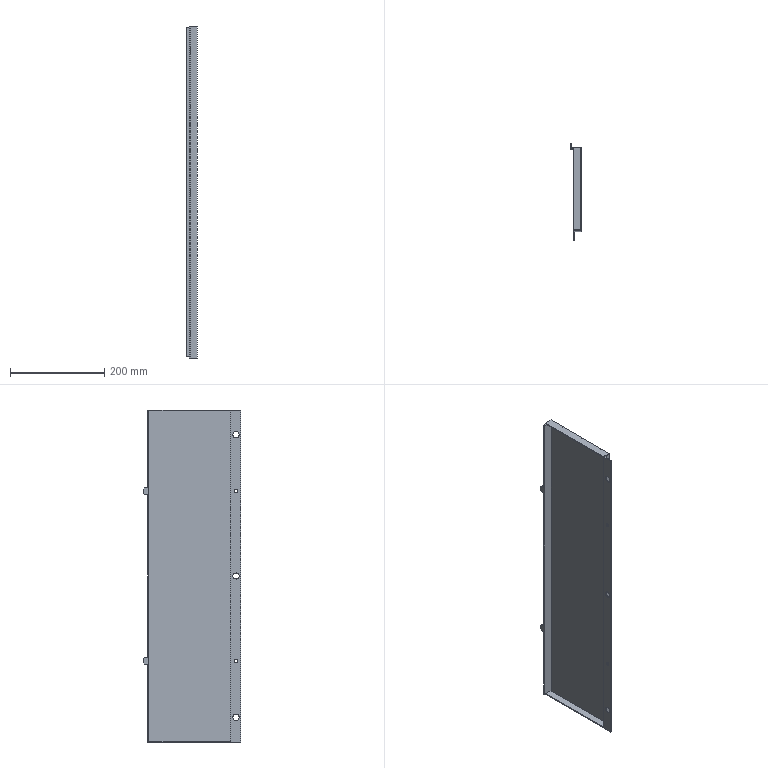Part | SolidWorks | features BaseBody 1 | 1 solid | 42 faces | box 22 x 207 x 705 mm | volume 336942 mm3 | plane 32 | cylinder 10 | commonest cylinder face diameters 13.1 x6 7.2 x4
STEP:
#1=CARTESIAN_POINT('',(194.446,-4330.973,1546.371));
#2=VERTEX_POINT('',#1);
#3=CARTESIAN_POINT('',(194.446,-4330.973,1553.571));
#4=VERTEX_POINT('',#3);
#5=CARTESIAN_POINT('',(194.446,-4330.973,1549.971));
#6=DIRECTION('',(-1.,0.,0.));
#7=DIRECTION('',(0.,0.,1.));
#8=AXIS2_PLACEMENT_3D('',#5,#6,#7);
#9=CIRCLE('',#8,3.6);
#10=EDGE_CURVE('',#2,#4,#9,.T.);
#11=ORIENTED_EDGE('',*,*,#10,.F.);
#12=CARTESIAN_POINT('',(192.446,-4330.973,1546.371));
#13=VERTEX_POINT('',#12);
#14=CARTESIAN_POINT('',(201.592,-4330.973,1546.371));
#15=DIRECTION('',(-1.,0.,0.));
#16=VECTOR('',#15,1000.);
#17=LINE('',#14,#16);
#18=EDGE_CURVE('',#2,#13,#17,.T.);
#19=ORIENTED_EDGE('',*,*,#18,.T.);
#20=CARTESIAN_POINT('',(192.446,-4330.973,1553.571));
#21=VERTEX_POINT('',#20);
#22=CARTESIAN_POINT('',(192.446,-4330.973,1549.971));
#23=DIRECTION('',(1.,0.,0.));
#24=DIRECTION('',(0.,0.,1.));
#25=AXIS2_PLACEMENT_3D('',#22,#23,#24);
#26=CIRCLE('',#25,3.6);
#27=EDGE_CURVE('',#21,#13,#26,.T.);
#28=ORIENTED_EDGE('',*,*,#27,.F.);
#29=CARTESIAN_POINT('',(201.592,-4330.973,1553.571));
#30=DIRECTION('',(-1.,0.,0.));
#31=VECTOR('',#30,1000.);
#32=LINE('',#29,#31);
#33=EDGE_CURVE('',#4,#21,#32,.T.);
#34=ORIENTED_EDGE('',*,*,#33,.F.);
#35=EDGE_LOOP('',(#11,#19,#28,#34));
#36=FACE_OUTER_BOUND('',#35,.T.);
#37=CARTESIAN_POINT('',(201.592,-4330.973,1549.971));
#38=DIRECTION('',(-1.,0.,0.));
#39=DIRECTION('',(0.,0.,1.));
#40=AXIS2_PLACEMENT_3D('',#37,#38,#39);
#41=CYLINDRICAL_SURFACE('',#40,3.6);
#42=ADVANCED_FACE('',(#36),#41,.F.);
#43=CARTESIAN_POINT('',(194.446,-4330.973,1186.371));
#44=VERTEX_POINT('',#43);
#45=CARTESIAN_POINT('',(194.446,-4330.973,1193.571));
#46=VERTEX_POINT('',#45);
#47=CARTESIAN_POINT('',(194.446,-4330.973,1189.971));
#48=DIRECTION('',(-1.,0.,0.));
#49=DIRECTION('',(0.,0.,1.));
#50=AXIS2_PLACEMENT_3D('',#47,#48,#49);
#51=CIRCLE('',#50,3.6);
#52=EDGE_CURVE('',#44,#46,#51,.T.);
#53=ORIENTED_EDGE('',*,*,#52,.F.);
#54=CARTESIAN_POINT('',(192.446,-4330.973,1186.371));
#55=VERTEX_POINT('',#54);
#56=CARTESIAN_POINT('',(201.592,-4330.973,1186.371));
#57=DIRECTION('',(-1.,0.,0.));
#58=VECTOR('',#57,1000.);
#59=LINE('',#56,#58);
#60=EDGE_CURVE('',#44,#55,#59,.T.);
#61=ORIENTED_EDGE('',*,*,#60,.T.);
#62=CARTESIAN_POINT('',(192.446,-4330.973,1193.571));
#63=VERTEX_POINT('',#62);
#64=CARTESIAN_POINT('',(192.446,-4330.973,1189.971));
#65=DIRECTION('',(1.,0.,0.));
#66=DIRECTION('',(0.,0.,1.));
#67=AXIS2_PLACEMENT_3D('',#64,#65,#66);
#68=CIRCLE('',#67,3.6);
#69=EDGE_CURVE('',#63,#55,#68,.T.);
#70=ORIENTED_EDGE('',*,*,#69,.F.);
#71=CARTESIAN_POINT('',(201.592,-4330.973,1193.571));
#72=DIRECTION('',(-1.,0.,0.));
#73=VECTOR('',#72,1000.);
#74=LINE('',#71,#73);
#75=EDGE_CURVE('',#46,#63,#74,.T.);
#76=ORIENTED_EDGE('',*,*,#75,.F.);
#77=EDGE_LOOP('',(#53,#61,#70,#76));
#78=FACE_OUTER_BOUND('',#77,.T.);
#79=CARTESIAN_POINT('',(201.592,-4330.973,1189.971));
#80=DIRECTION('',(-1.,0.,0.));
#81=DIRECTION('',(0.,0.,1.));
#82=AXIS2_PLACEMENT_3D('',#79,#80,#81);
#83=CYLINDRICAL_SURFACE('',#82,3.6);
#84=ADVANCED_FACE('',(#78),#83,.F.);
#85=CARTESIAN_POINT('',(194.446,-4330.973,1063.421));
#86=VERTEX_POINT('',#85);
#87=CARTESIAN_POINT('',(194.446,-4330.973,1076.521));
#88=VERTEX_POINT('',#87);
#89=CARTESIAN_POINT('',(194.446,-4330.973,1069.971));
#90=DIRECTION('',(-1.,0.,0.));
#91=DIRECTION('',(0.,0.,1.));
#92=AXIS2_PLACEMENT_3D('',#89,#90,#91);
#93=CIRCLE('',#92,6.55);
#94=EDGE_CURVE('',#86,#88,#93,.T.);
#95=ORIENTED_EDGE('',*,*,#94,.F.);
#96=CARTESIAN_POINT('',(192.446,-4330.973,1063.421));
#97=VERTEX_POINT('',#96);
#98=CARTESIAN_POINT('',(194.687,-4330.973,1063.421));
#99=DIRECTION('',(-1.,0.,0.));
#100=VECTOR('',#99,1000.);
#101=LINE('',#98,#100);
#102=EDGE_CURVE('',#86,#97,#101,.T.);
#103=ORIENTED_EDGE('',*,*,#102,.T.);
#104=CARTESIAN_POINT('',(192.446,-4330.973,1076.521));
#105=VERTEX_POINT('',#104);
#106=CARTESIAN_POINT('',(192.446,-4330.973,1069.971));
#107=DIRECTION('',(1.,0.,0.));
#108=DIRECTION('',(0.,0.,1.));
#109=AXIS2_PLACEMENT_3D('',#106,#107,#108);
#110=CIRCLE('',#109,6.55);
#111=EDGE_CURVE('',#105,#97,#110,.T.);
#112=ORIENTED_EDGE('',*,*,#111,.F.);
#113=CARTESIAN_POINT('',(194.687,-4330.973,1076.521));
#114=DIRECTION('',(-1.,0.,0.));
#115=VECTOR('',#114,1000.);
#116=LINE('',#113,#115);
#117=EDGE_CURVE('',#88,#105,#116,.T.);
#118=ORIENTED_EDGE('',*,*,#117,.F.);
#119=EDGE_LOOP('',(#95,#103,#112,#118));
#120=FACE_OUTER_BOUND('',#119,.T.);
#121=CARTESIAN_POINT('',(194.687,-4330.973,1069.971));
#122=DIRECTION('',(-1.,0.,0.));
#123=DIRECTION('',(0.,0.,1.));
#124=AXIS2_PLACEMENT_3D('',#121,#122,#123);
#125=CYLINDRICAL_SURFACE('',#124,6.55);
#126=ADVANCED_FACE('',(#120),#125,.F.);
#127=CARTESIAN_POINT('',(194.446,-4330.973,1663.421));
#128=VERTEX_POINT('',#127);
#129=CARTESIAN_POINT('',(194.446,-4330.973,1676.521));
#130=VERTEX_POINT('',#129);
#131=CARTESIAN_POINT('',(194.446,-4330.973,1669.971));
#132=DIRECTION('',(-1.,0.,0.));
#133=DIRECTION('',(0.,0.,1.));
#134=AXIS2_PLACEMENT_3D('',#131,#132,#133);
#135=CIRCLE('',#134,6.55);
#136=EDGE_CURVE('',#128,#130,#135,.T.);
#137=ORIENTED_EDGE('',*,*,#136,.F.);
#138=CARTESIAN_POINT('',(192.446,-4330.973,1663.421));
#139=VERTEX_POINT('',#138);
#140=CARTESIAN_POINT('',(184.109,-4330.973,1663.421));
#141=DIRECTION('',(-1.,0.,0.));
#142=VECTOR('',#141,1000.);
#143=LINE('',#140,#142);
#144=EDGE_CURVE('',#128,#139,#143,.T.);
#145=ORIENTED_EDGE('',*,*,#144,.T.);
#146=CARTESIAN_POINT('',(192.446,-4330.973,1676.521));
#147=VERTEX_POINT('',#146);
#148=CARTESIAN_POINT('',(192.446,-4330.973,1669.971));
#149=DIRECTION('',(1.,0.,0.));
#150=DIRECTION('',(0.,0.,1.));
#151=AXIS2_PLACEMENT_3D('',#148,#149,#150);
#152=CIRCLE('',#151,6.55);
#153=EDGE_CURVE('',#147,#139,#152,.T.);
#154=ORIENTED_EDGE('',*,*,#153,.F.);
#155=CARTESIAN_POINT('',(184.109,-4330.973,1676.521));
#156=DIRECTION('',(-1.,0.,0.));
#157=VECTOR('',#156,1000.);
#158=LINE('',#155,#157);
#159=EDGE_CURVE('',#130,#147,#158,.T.);
#160=ORIENTED_EDGE('',*,*,#159,.F.);
#161=EDGE_LOOP('',(#137,#145,#154,#160));
#162=FACE_OUTER_BOUND('',#161,.T.);
#163=CARTESIAN_POINT('',(184.109,-4330.973,1669.971));
#164=DIRECTION('',(-1.,0.,0.));
#165=DIRECTION('',(0.,0.,1.));
#166=AXIS2_PLACEMENT_3D('',#163,#164,#165);
#167=CYLINDRICAL_SURFACE('',#166,6.55);
#168=ADVANCED_FACE('',(#162),#167,.F.);
#169=CARTESIAN_POINT('',(194.446,-4330.973,1363.421));
#170=VERTEX_POINT('',#169);
#171=CARTESIAN_POINT('',(194.446,-4330.973,1376.521));
#172=VERTEX_POINT('',#171);
#173=CARTESIAN_POINT('',(194.446,-4330.973,1369.971));
#174=DIRECTION('',(-1.,0.,0.));
#175=DIRECTION('',(0.,0.,1.));
#176=AXIS2_PLACEMENT_3D('',#173,#174,#175);
#177=CIRCLE('',#176,6.55);
#178=EDGE_CURVE('',#170,#172,#177,.T.);
#179=ORIENTED_EDGE('',*,*,#178,.F.);
#180=CARTESIAN_POINT('',(192.446,-4330.973,1363.421));
#181=VERTEX_POINT('',#180);
#182=CARTESIAN_POINT('',(194.687,-4330.973,1363.421));
#183=DIRECTION('',(-1.,0.,0.));
#184=VECTOR('',#183,1000.);
#185=LINE('',#182,#184);
#186=EDGE_CURVE('',#170,#181,#185,.T.);
#187=ORIENTED_EDGE('',*,*,#186,.T.);
#188=CARTESIAN_POINT('',(192.446,-4330.973,1376.521));
#189=VERTEX_POINT('',#188);
#190=CARTESIAN_POINT('',(192.446,-4330.973,1369.971));
#191=DIRECTION('',(1.,0.,0.));
#192=DIRECTION('',(0.,0.,1.));
#193=AXIS2_PLACEMENT_3D('',#190,#191,#192);
#194=CIRCLE('',#193,6.55);
#195=EDGE_CURVE('',#189,#181,#194,.T.);
#196=ORIENTED_EDGE('',*,*,#195,.F.);
#197=CARTESIAN_POINT('',(194.687,-4330.973,1376.521));
#198=DIRECTION('',(-1.,0.,0.));
#199=VECTOR('',#198,1000.);
#200=LINE('',#197,#199);
#201=EDGE_CURVE('',#172,#189,#200,.T.);
#202=ORIENTED_EDGE('',*,*,#201,.F.);
#203=EDGE_LOOP('',(#179,#187,#196,#202));
#204=FACE_OUTER_BOUND('',#203,.T.);
#205=CARTESIAN_POINT('',(194.687,-4330.973,1369.971));
#206=DIRECTION('',(-1.,0.,0.));
#207=DIRECTION('',(0.,0.,1.));
#208=AXIS2_PLACEMENT_3D('',#205,#206,#207);
#209=CYLINDRICAL_SURFACE('',#208,6.55);
#210=ADVANCED_FACE('',(#204),#209,.F.);
#211=CARTESIAN_POINT('',(209.446,-4320.973,1017.471));
#212=VERTEX_POINT('',#211);
#213=CARTESIAN_POINT('',(209.446,-4143.973,1017.471));
#214=VERTEX_POINT('',#213);
#215=CARTESIAN_POINT('',(209.446,-4143.973,1017.471));
#216=DIRECTION('',(0.,1.,0.));
#217=VECTOR('',#216,1000.);
#218=LINE('',#215,#217);
#219=EDGE_CURVE('',#212,#214,#218,.T.);
#220=ORIENTED_EDGE('',*,*,#219,.T.);
#221=CARTESIAN_POINT('',(209.446,-4143.973,1722.471));
#222=VERTEX_POINT('',#221);
#223=CARTESIAN_POINT('',(209.446,-4143.973,1017.471));
#224=DIRECTION('',(0.,0.,1.));
#225=VECTOR('',#224,1000.);
#226=LINE('',#223,#225);
#227=EDGE_CURVE('',#214,#222,#226,.T.);
#228=ORIENTED_EDGE('',*,*,#227,.T.);
#229=CARTESIAN_POINT('',(209.446,-4320.973,1722.471));
#230=VERTEX_POINT('',#229);
#231=CARTESIAN_POINT('',(209.446,-4143.973,1722.471));
#232=DIRECTION('',(0.,-1.,0.));
#233=VECTOR('',#232,1000.);
#234=LINE('',#231,#233);
#235=EDGE_CURVE('',#222,#230,#234,.T.);
#236=ORIENTED_EDGE('',*,*,#235,.T.);
#237=CARTESIAN_POINT('',(209.446,-4320.973,1017.471));
#238=DIRECTION('',(0.,0.,-1.));
#239=VECTOR('',#238,1000.);
#240=LINE('',#237,#239);
#241=EDGE_CURVE('',#230,#212,#240,.T.);
#242=ORIENTED_EDGE('',*,*,#241,.T.);
#243=EDGE_LOOP('',(#220,#228,#236,#242));
#244=FACE_OUTER_BOUND('',#243,.T.);
#245=CARTESIAN_POINT('',(209.446,-4143.973,1017.471));
#246=DIRECTION('',(1.,0.,0.));
#247=DIRECTION('',(0.,0.,-1.));
#248=AXIS2_PLACEMENT_3D('',#245,#246,#247);
#249=PLANE('',#248);
#250=ADVANCED_FACE('',(#244),#249,.T.);
#251=CARTESIAN_POINT('',(187.446,-4143.973,1182.471));
#252=VERTEX_POINT('',#251);
#253=CARTESIAN_POINT('',(189.446,-4143.973,1182.471));
#254=VERTEX_POINT('',#253);
#255=CARTESIAN_POINT('',(207.446,-4143.973,1182.471));
#256=DIRECTION('',(1.,0.,0.));
#257=VECTOR('',#256,1000.);
#258=LINE('',#255,#257);
#259=EDGE_CURVE('',#252,#254,#258,.T.);
#260=ORIENTED_EDGE('',*,*,#259,.T.);
#261=CARTESIAN_POINT('',(189.446,-4143.973,1197.471));
#262=VERTEX_POINT('',#261);
#263=CARTESIAN_POINT('',(189.446,-4143.973,1720.471));
#264=DIRECTION('',(0.,0.,1.));
#265=VECTOR('',#264,1000.);
#266=LINE('',#263,#265);
#267=EDGE_CURVE('',#254,#262,#266,.T.);
#268=ORIENTED_EDGE('',*,*,#267,.T.);
#269=CARTESIAN_POINT('',(187.446,-4143.973,1197.471));
#270=VERTEX_POINT('',#269);
#271=CARTESIAN_POINT('',(207.446,-4143.973,1197.471));
#272=DIRECTION('',(-1.,0.,0.));
#273=VECTOR('',#272,1000.);
#274=LINE('',#271,#273);
#275=EDGE_CURVE('',#262,#270,#274,.T.);
#276=ORIENTED_EDGE('',*,*,#275,.T.);
#277=CARTESIAN_POINT('',(187.446,-4143.973,1542.471));
#278=VERTEX_POINT('',#277);
#279=CARTESIAN_POINT('',(187.446,-4143.973,1720.471));
#280=DIRECTION('',(0.,0.,1.));
#281=VECTOR('',#280,1000.);
#282=LINE('',#279,#281);
#283=EDGE_CURVE('',#270,#278,#282,.T.);
#284=ORIENTED_EDGE('',*,*,#283,.T.);
#285=CARTESIAN_POINT('',(189.446,-4143.973,1542.471));
#286=VERTEX_POINT('',#285);
#287=CARTESIAN_POINT('',(207.446,-4143.973,1542.471));
#288=DIRECTION('',(1.,0.,0.));
#289=VECTOR('',#288,1000.);
#290=LINE('',#287,#289);
#291=EDGE_CURVE('',#278,#286,#290,.T.);
#292=ORIENTED_EDGE('',*,*,#291,.T.);
#293=CARTESIAN_POINT('',(189.446,-4143.973,1557.471));
#294=VERTEX_POINT('',#293);
#295=CARTESIAN_POINT('',(189.446,-4143.973,1720.471));
#296=DIRECTION('',(0.,0.,1.));
#297=VECTOR('',#296,1000.);
#298=LINE('',#295,#297);
#299=EDGE_CURVE('',#286,#294,#298,.T.);
#300=ORIENTED_EDGE('',*,*,#299,.T.);
#301=CARTESIAN_POINT('',(187.446,-4143.973,1557.471));
#302=VERTEX_POINT('',#301);
#303=CARTESIAN_POINT('',(207.446,-4143.973,1557.471));
#304=DIRECTION('',(-1.,0.,0.));
#305=VECTOR('',#304,1000.);
#306=LINE('',#303,#305);
#307=EDGE_CURVE('',#294,#302,#306,.T.);
#308=ORIENTED_EDGE('',*,*,#307,.T.);
#309=CARTESIAN_POINT('',(187.446,-4143.973,1719.471));
#310=VERTEX_POINT('',#309);
#311=CARTESIAN_POINT('',(187.446,-4143.973,1720.471));
#312=DIRECTION('',(0.,0.,1.));
#313=VECTOR('',#312,1000.);
#314=LINE('',#311,#313);
#315=EDGE_CURVE('',#302,#310,#314,.T.);
#316=ORIENTED_EDGE('',*,*,#315,.T.);
#317=CARTESIAN_POINT('',(207.446,-4143.973,1719.471));
#318=VERTEX_POINT('',#317);
#319=CARTESIAN_POINT('',(207.446,-4143.973,1719.471));
#320=DIRECTION('',(1.,0.,0.));
#321=VECTOR('',#320,1000.);
#322=LINE('',#319,#321);
#323=EDGE_CURVE('',#310,#318,#322,.T.);
#324=ORIENTED_EDGE('',*,*,#323,.T.);
#325=CARTESIAN_POINT('',(207.446,-4143.973,1720.471));
#326=VERTEX_POINT('',#325);
#327=CARTESIAN_POINT('',(207.446,-4143.973,1017.471));
#328=DIRECTION('',(0.,0.,-1.));
#329=VECTOR('',#328,1000.);
#330=LINE('',#327,#329);
#331=EDGE_CURVE('',#326,#318,#330,.T.);
#332=ORIENTED_EDGE('',*,*,#331,.F.);
#333=CARTESIAN_POINT('',(192.446,-4143.973,1720.471));
#334=VERTEX_POINT('',#333);
#335=CARTESIAN_POINT('',(207.446,-4143.973,1720.471));
#336=DIRECTION('',(-1.,0.,0.));
#337=VECTOR('',#336,1000.);
#338=LINE('',#335,#337);
#339=EDGE_CURVE('',#326,#334,#338,.T.);
#340=ORIENTED_EDGE('',*,*,#339,.T.);
#341=CARTESIAN_POINT('',(192.446,-4143.973,1722.471));
#342=VERTEX_POINT('',#341);
#343=CARTESIAN_POINT('',(192.446,-4143.973,1720.471));
#344=DIRECTION('',(0.,0.,1.));
#345=VECTOR('',#344,1000.);
#346=LINE('',#343,#345);
#347=EDGE_CURVE('',#334,#342,#346,.T.);
#348=ORIENTED_EDGE('',*,*,#347,.T.);
#349=CARTESIAN_POINT('',(207.446,-4143.973,1722.471));
#350=DIRECTION('',(1.,0.,0.));
#351=VECTOR('',#350,1000.);
#352=LINE('',#349,#351);
#353=EDGE_CURVE('',#342,#222,#352,.T.);
#354=ORIENTED_EDGE('',*,*,#353,.T.);
#355=ORIENTED_EDGE('',*,*,#227,.F.);
#356=CARTESIAN_POINT('',(192.446,-4143.973,1017.471));
#357=VERTEX_POINT('',#356);
#358=CARTESIAN_POINT('',(207.446,-4143.973,1017.471));
#359=DIRECTION('',(-1.,0.,0.));
#360=VECTOR('',#359,1000.);
#361=LINE('',#358,#360);
#362=EDGE_CURVE('',#214,#357,#361,.T.);
#363=ORIENTED_EDGE('',*,*,#362,.T.);
#364=CARTESIAN_POINT('',(192.446,-4143.973,1019.471));
#365=VERTEX_POINT('',#364);
#366=CARTESIAN_POINT('',(192.446,-4143.973,1720.471));
#367=DIRECTION('',(0.,0.,1.));
#368=VECTOR('',#367,1000.);
#369=LINE('',#366,#368);
#370=EDGE_CURVE('',#357,#365,#369,.T.);
#371=ORIENTED_EDGE('',*,*,#370,.T.);
#372=CARTESIAN_POINT('',(207.446,-4143.973,1019.471));
#373=VERTEX_POINT('',#372);
#374=CARTESIAN_POINT('',(207.446,-4143.973,1019.471));
#375=DIRECTION('',(1.,0.,0.));
#376=VECTOR('',#375,1000.);
#377=LINE('',#374,#376);
#378=EDGE_CURVE('',#365,#373,#377,.T.);
#379=ORIENTED_EDGE('',*,*,#378,.T.);
#380=CARTESIAN_POINT('',(207.446,-4143.973,1020.471));
#381=VERTEX_POINT('',#380);
#382=CARTESIAN_POINT('',(207.446,-4143.973,1017.471));
#383=DIRECTION('',(0.,0.,-1.));
#384=VECTOR('',#383,1000.);
#385=LINE('',#382,#384);
#386=EDGE_CURVE('',#381,#373,#385,.T.);
#387=ORIENTED_EDGE('',*,*,#386,.F.);
#388=CARTESIAN_POINT('',(187.446,-4143.973,1020.471));
#389=VERTEX_POINT('',#388);
#390=CARTESIAN_POINT('',(207.446,-4143.973,1020.471));
#391=DIRECTION('',(-1.,0.,0.));
#392=VECTOR('',#391,1000.);
#393=LINE('',#390,#392);
#394=EDGE_CURVE('',#381,#389,#393,.T.);
#395=ORIENTED_EDGE('',*,*,#394,.T.);
#396=CARTESIAN_POINT('',(187.446,-4143.973,1720.471));
#397=DIRECTION('',(0.,0.,1.));
#398=VECTOR('',#397,1000.);
#399=LINE('',#396,#398);
#400=EDGE_CURVE('',#389,#252,#399,.T.);
#401=ORIENTED_EDGE('',*,*,#400,.T.);
#402=EDGE_LOOP('',(#260,#268,#276,#284,#292,#300,#308,#316,#324,#332,#340,#348,#354,#355,#363,#371,#379,#387,#395,#401));
#403=FACE_OUTER_BOUND('',#402,.T.);
#404=CARTESIAN_POINT('',(207.446,-4143.973,1720.471));
#405=DIRECTION('',(0.,1.,0.));
#406=DIRECTION('',(0.,0.,1.));
#407=AXIS2_PLACEMENT_3D('',#404,#405,#406);
#408=PLANE('',#407);
#409=ADVANCED_FACE('',(#403),#408,.T.);
#410=CARTESIAN_POINT('',(207.446,-4318.473,1017.471));
#411=VERTEX_POINT('',#410);
#412=CARTESIAN_POINT('',(207.446,-4318.973,1017.471));
#413=VERTEX_POINT('',#412);
#414=CARTESIAN_POINT('',(207.446,-4318.973,1017.471));
#415=DIRECTION('',(0.,-1.,0.));
#416=VECTOR('',#415,1000.);
#417=LINE('',#414,#416);
#418=EDGE_CURVE('',#411,#413,#417,.T.);
#419=ORIENTED_EDGE('',*,*,#418,.F.);
#420=CARTESIAN_POINT('',(192.446,-4318.473,1017.471));
#421=VERTEX_POINT('',#420);
#422=CARTESIAN_POINT('',(207.446,-4318.473,1017.471));
#423=DIRECTION('',(-1.,0.,0.));
#424=VECTOR('',#423,1000.);
#425=LINE('',#422,#424);
#426=EDGE_CURVE('',#411,#421,#425,.T.);
#427=ORIENTED_EDGE('',*,*,#426,.T.);
#428=CARTESIAN_POINT('',(192.446,-4143.973,1017.471));
#429=DIRECTION('',(0.,1.,0.));
#430=VECTOR('',#429,1000.);
#431=LINE('',#428,#430);
#432=EDGE_CURVE('',#421,#357,#431,.T.);
#433=ORIENTED_EDGE('',*,*,#432,.T.);
#434=ORIENTED_EDGE('',*,*,#362,.F.);
#435=ORIENTED_EDGE('',*,*,#219,.F.);
#436=CARTESIAN_POINT('',(194.446,-4320.973,1017.471));
#437=VERTEX_POINT('',#436);
#438=CARTESIAN_POINT('',(207.446,-4320.973,1017.471));
#439=DIRECTION('',(-1.,0.,0.));
#440=VECTOR('',#439,1000.);
#441=LINE('',#438,#440);
#442=EDGE_CURVE('',#212,#437,#441,.T.);
#443=ORIENTED_EDGE('',*,*,#442,.T.);
#444=CARTESIAN_POINT('',(194.446,-4340.973,1017.471));
#445=VERTEX_POINT('',#444);
#446=CARTESIAN_POINT('',(194.446,-4143.973,1017.471));
#447=DIRECTION('',(0.,-1.,0.));
#448=VECTOR('',#447,1000.);
#449=LINE('',#446,#448);
#450=EDGE_CURVE('',#437,#445,#449,.T.);
#451=ORIENTED_EDGE('',*,*,#450,.T.);
#452=CARTESIAN_POINT('',(192.446,-4340.973,1017.471));
#453=VERTEX_POINT('',#452);
#454=CARTESIAN_POINT('',(207.446,-4340.973,1017.471));
#455=DIRECTION('',(-1.,0.,0.));
#456=VECTOR('',#455,1000.);
#457=LINE('',#454,#456);
#458=EDGE_CURVE('',#445,#453,#457,.T.);
#459=ORIENTED_EDGE('',*,*,#458,.T.);
#460=CARTESIAN_POINT('',(192.446,-4318.973,1017.471));
#461=VERTEX_POINT('',#460);
#462=CARTESIAN_POINT('',(192.446,-4143.973,1017.471));
#463=DIRECTION('',(0.,1.,0.));
#464=VECTOR('',#463,1000.);
#465=LINE('',#462,#464);
#466=EDGE_CURVE('',#453,#461,#465,.T.);
#467=ORIENTED_EDGE('',*,*,#466,.T.);
#468=CARTESIAN_POINT('',(207.446,-4318.973,1017.471));
#469=DIRECTION('',(1.,0.,0.));
#470=VECTOR('',#469,1000.);
#471=LINE('',#468,#470);
#472=EDGE_CURVE('',#461,#413,#471,.T.);
#473=ORIENTED_EDGE('',*,*,#472,.T.);
#474=EDGE_LOOP('',(#419,#427,#433,#434,#435,#443,#451,#459,#467,#473));
#475=FACE_OUTER_BOUND('',#474,.T.);
#476=CARTESIAN_POINT('',(207.446,-4143.973,1017.471));
#477=DIRECTION('',(0.,0.,-1.));
#478=DIRECTION('',(-1.,0.,0.));
#479=AXIS2_PLACEMENT_3D('',#476,#477,#478);
#480=PLANE('',#479);
#481=ADVANCED_FACE('',(#475),#480,.T.);
#482=ORIENTED_EDGE('',*,*,#442,.F.);
#483=ORIENTED_EDGE('',*,*,#241,.F.);
#484=CARTESIAN_POINT('',(194.446,-4320.973,1722.471));
#485=VERTEX_POINT('',#484);
#486=CARTESIAN_POINT('',(209.446,-4320.973,1722.471));
#487=DIRECTION('',(-1.,0.,0.));
#488=VECTOR('',#487,1000.);
#489=LINE('',#486,#488);
#490=EDGE_CURVE('',#230,#485,#489,.T.);
#491=ORIENTED_EDGE('',*,*,#490,.T.);
#492=CARTESIAN_POINT('',(194.446,-4320.973,1017.471));
#493=DIRECTION('',(0.,0.,-1.));
#494=VECTOR('',#493,1000.);
#495=LINE('',#492,#494);
#496=EDGE_CURVE('',#485,#437,#495,.T.);
#497=ORIENTED_EDGE('',*,*,#496,.T.);
#498=EDGE_LOOP('',(#482,#483,#491,#497));
#499=FACE_OUTER_BOUND('',#498,.T.);
#500=CARTESIAN_POINT('',(209.446,-4320.973,1017.471));
#501=DIRECTION('',(0.,-1.,0.));
#502=DIRECTION('',(0.,0.,-1.));
#503=AXIS2_PLACEMENT_3D('',#500,#501,#502);
#504=PLANE('',#503);
#505=ADVANCED_FACE('',(#499),#504,.T.);
#506=ORIENTED_EDGE('',*,*,#235,.F.);
#507=ORIENTED_EDGE('',*,*,#353,.F.);
#508=CARTESIAN_POINT('',(192.446,-4318.473,1722.471));
#509=VERTEX_POINT('',#508);
#510=CARTESIAN_POINT('',(192.446,-4143.973,1722.471));
#511=DIRECTION('',(0.,-1.,0.));
#512=VECTOR('',#511,1000.);
#513=LINE('',#510,#512);
#514=EDGE_CURVE('',#342,#509,#513,.T.);
#515=ORIENTED_EDGE('',*,*,#514,.T.);
#516=CARTESIAN_POINT('',(207.446,-4318.473,1722.471));
#517=VERTEX_POINT('',#516);
#518=CARTESIAN_POINT('',(207.446,-4318.473,1722.471));
#519=DIRECTION('',(1.,0.,0.));
#520=VECTOR('',#519,1000.);
#521=LINE('',#518,#520);
#522=EDGE_CURVE('',#509,#517,#521,.T.);
#523=ORIENTED_EDGE('',*,*,#522,.T.);
#524=CARTESIAN_POINT('',(207.446,-4318.973,1722.471));
#525=VERTEX_POINT('',#524);
#526=CARTESIAN_POINT('',(207.446,-4318.973,1722.471));
#527=DIRECTION('',(0.,1.,0.));
#528=VECTOR('',#527,1000.);
#529=LINE('',#526,#528);
#530=EDGE_CURVE('',#525,#517,#529,.T.);
#531=ORIENTED_EDGE('',*,*,#530,.F.);
#532=CARTESIAN_POINT('',(192.446,-4318.973,1722.471));
#533=VERTEX_POINT('',#532);
#534=CARTESIAN_POINT('',(207.446,-4318.973,1722.471));
#535=DIRECTION('',(-1.,0.,0.));
#536=VECTOR('',#535,1000.);
#537=LINE('',#534,#536);
#538=EDGE_CURVE('',#525,#533,#537,.T.);
#539=ORIENTED_EDGE('',*,*,#538,.T.);
#540=CARTESIAN_POINT('',(192.446,-4340.973,1722.471));
#541=VERTEX_POINT('',#540);
#542=CARTESIAN_POINT('',(192.446,-4143.973,1722.471));
#543=DIRECTION('',(0.,-1.,0.));
#544=VECTOR('',#543,1000.);
#545=LINE('',#542,#544);
#546=EDGE_CURVE('',#533,#541,#545,.T.);
#547=ORIENTED_EDGE('',*,*,#546,.T.);
#548=CARTESIAN_POINT('',(194.446,-4340.973,1722.471));
#549=VERTEX_POINT('',#548);
#550=CARTESIAN_POINT('',(207.446,-4340.973,1722.471));
#551=DIRECTION('',(1.,0.,0.));
#552=VECTOR('',#551,1000.);
#553=LINE('',#550,#552);
#554=EDGE_CURVE('',#541,#549,#553,.T.);
#555=ORIENTED_EDGE('',*,*,#554,.T.);
#556=CARTESIAN_POINT('',(194.446,-4143.973,1722.471));
#557=DIRECTION('',(0.,1.,0.));
#558=VECTOR('',#557,1000.);
#559=LINE('',#556,#558);
#560=EDGE_CURVE('',#549,#485,#559,.T.);
#561=ORIENTED_EDGE('',*,*,#560,.T.);
#562=ORIENTED_EDGE('',*,*,#490,.F.);
#563=EDGE_LOOP('',(#506,#507,#515,#523,#531,#539,#547,#555,#561,#562));
#564=FACE_OUTER_BOUND('',#563,.T.);
#565=CARTESIAN_POINT('',(207.446,-4143.973,1722.471));
#566=DIRECTION('',(0.,0.,1.));
#567=DIRECTION('',(1.,0.,0.));
#568=AXIS2_PLACEMENT_3D('',#565,#566,#567);
#569=PLANE('',#568);
#570=ADVANCED_FACE('',(#564),#569,.T.);
#571=CARTESIAN_POINT('',(189.446,-4133.973,1194.471));
#572=VERTEX_POINT('',#571);
#573=CARTESIAN_POINT('',(189.446,-4136.973,1197.471));
#574=VERTEX_POINT('',#573);
#575=CARTESIAN_POINT('',(189.446,-4133.973,1194.471));
#576=DIRECTION('',(0.,-0.7071,0.7071));
#577=VECTOR('',#576,1000.);
#578=LINE('',#575,#577);
#579=EDGE_CURVE('',#572,#574,#578,.T.);
#580=ORIENTED_EDGE('',*,*,#579,.T.);
#581=CARTESIAN_POINT('',(189.446,-4140.465,1197.471));
#582=DIRECTION('',(0.,-1.,0.));
#583=VECTOR('',#582,1000.);
#584=LINE('',#581,#583);
#585=EDGE_CURVE('',#574,#262,#584,.T.);
#586=ORIENTED_EDGE('',*,*,#585,.T.);
#587=ORIENTED_EDGE('',*,*,#267,.F.);
#588=CARTESIAN_POINT('',(189.446,-4136.973,1182.471));
#589=VERTEX_POINT('',#588);
#590=CARTESIAN_POINT('',(189.446,-4140.465,1182.471));
#591=DIRECTION('',(0.,1.,0.));
#592=VECTOR('',#591,1000.);
#593=LINE('',#590,#592);
#594=EDGE_CURVE('',#254,#589,#593,.T.);
#595=ORIENTED_EDGE('',*,*,#594,.T.);
#596=CARTESIAN_POINT('',(189.446,-4133.973,1185.471));
#597=VERTEX_POINT('',#596);
#598=CARTESIAN_POINT('',(189.446,-4136.973,1182.471));
#599=DIRECTION('',(0.,0.7071,0.7071));
#600=VECTOR('',#599,1000.);
#601=LINE('',#598,#600);
#602=EDGE_CURVE('',#589,#597,#601,.T.);
#603=ORIENTED_EDGE('',*,*,#602,.T.);
#604=CARTESIAN_POINT('',(189.446,-4133.973,1189.971));
#605=DIRECTION('',(0.,0.,1.));
#606=VECTOR('',#605,1000.);
#607=LINE('',#604,#606);
#608=EDGE_CURVE('',#597,#572,#607,.T.);
#609=ORIENTED_EDGE('',*,*,#608,.T.);
#610=EDGE_LOOP('',(#580,#586,#587,#595,#603,#609));
#611=FACE_OUTER_BOUND('',#610,.T.);
#612=CARTESIAN_POINT('',(189.446,-4140.465,1189.971));
#613=DIRECTION('',(1.,0.,0.));
#614=DIRECTION('',(0.,0.,-1.));
#615=AXIS2_PLACEMENT_3D('',#612,#613,#614);
#616=PLANE('',#615);
#617=ADVANCED_FACE('',(#611),#616,.T.);
#618=CARTESIAN_POINT('',(187.446,-4136.973,1182.471));
#619=VERTEX_POINT('',#618);
#620=CARTESIAN_POINT('',(189.446,-4136.973,1182.471));
#621=DIRECTION('',(1.,0.,0.));
#622=VECTOR('',#621,1000.);
#623=LINE('',#620,#622);
#624=EDGE_CURVE('',#619,#589,#623,.T.);
#625=ORIENTED_EDGE('',*,*,#624,.T.);
#626=ORIENTED_EDGE('',*,*,#594,.F.);
#627=ORIENTED_EDGE('',*,*,#259,.F.);
#628=CARTESIAN_POINT('',(187.446,-4145.973,1182.471));
#629=DIRECTION('',(0.,1.,0.));
#630=VECTOR('',#629,1000.);
#631=LINE('',#628,#630);
#632=EDGE_CURVE('',#252,#619,#631,.T.);
#633=ORIENTED_EDGE('',*,*,#632,.T.);
#634=EDGE_LOOP('',(#625,#626,#627,#633));
#635=FACE_OUTER_BOUND('',#634,.T.);
#636=CARTESIAN_POINT('',(189.446,-4145.973,1182.471));
#637=DIRECTION('',(0.,0.,-1.));
#638=DIRECTION('',(-1.,0.,0.));
#639=AXIS2_PLACEMENT_3D('',#636,#637,#638);
#640=PLANE('',#639);
#641=ADVANCED_FACE('',(#635),#640,.T.);
#642=CARTESIAN_POINT('',(187.446,-4133.973,1194.471));
#643=VERTEX_POINT('',#642);
#644=CARTESIAN_POINT('',(187.446,-4136.973,1197.471));
#645=VERTEX_POINT('',#644);
#646=CARTESIAN_POINT('',(187.446,-4133.973,1194.471));
#647=DIRECTION('',(0.,-0.7071,0.7071));
#648=VECTOR('',#647,1000.);
#649=LINE('',#646,#648);
#650=EDGE_CURVE('',#643,#645,#649,.T.);
#651=ORIENTED_EDGE('',*,*,#650,.F.);
#652=CARTESIAN_POINT('',(187.446,-4133.973,1185.471));
#653=VERTEX_POINT('',#652);
#654=CARTESIAN_POINT('',(187.446,-4133.973,1189.971));
#655=DIRECTION('',(0.,0.,1.));
#656=VECTOR('',#655,1000.);
#657=LINE('',#654,#656);
#658=EDGE_CURVE('',#653,#643,#657,.T.);
#659=ORIENTED_EDGE('',*,*,#658,.F.);
#660=CARTESIAN_POINT('',(187.446,-4136.973,1182.471));
#661=DIRECTION('',(0.,0.7071,0.7071));
#662=VECTOR('',#661,1000.);
#663=LINE('',#660,#662);
#664=EDGE_CURVE('',#619,#653,#663,.T.);
#665=ORIENTED_EDGE('',*,*,#664,.F.);
#666=ORIENTED_EDGE('',*,*,#632,.F.);
#667=ORIENTED_EDGE('',*,*,#400,.F.);
#668=CARTESIAN_POINT('',(187.446,-4145.973,1020.471));
#669=VERTEX_POINT('',#668);
#670=CARTESIAN_POINT('',(187.446,-4140.465,1020.471));
#671=DIRECTION('',(0.,1.,0.));
#672=VECTOR('',#671,1000.);
#673=LINE('',#670,#672);
#674=EDGE_CURVE('',#669,#389,#673,.T.);
#675=ORIENTED_EDGE('',*,*,#674,.F.);
#676=CARTESIAN_POINT('',(187.446,-4145.973,1719.471));
#677=VERTEX_POINT('',#676);
#678=CARTESIAN_POINT('',(187.446,-4145.973,1189.971));
#679=DIRECTION('',(0.,0.,-1.));
#680=VECTOR('',#679,1000.);
#681=LINE('',#678,#680);
#682=EDGE_CURVE('',#677,#669,#681,.T.);
#683=ORIENTED_EDGE('',*,*,#682,.F.);
#684=CARTESIAN_POINT('',(187.446,-4140.465,1719.471));
#685=DIRECTION('',(0.,-1.,0.));
#686=VECTOR('',#685,1000.);
#687=LINE('',#684,#686);
#688=EDGE_CURVE('',#310,#677,#687,.T.);
#689=ORIENTED_EDGE('',*,*,#688,.F.);
#690=ORIENTED_EDGE('',*,*,#315,.F.);
#691=CARTESIAN_POINT('',(187.446,-4136.973,1557.471));
#692=VERTEX_POINT('',#691);
#693=CARTESIAN_POINT('',(187.446,-4140.465,1557.471));
#694=DIRECTION('',(0.,-1.,0.));
#695=VECTOR('',#694,1000.);
#696=LINE('',#693,#695);
#697=EDGE_CURVE('',#692,#302,#696,.T.);
#698=ORIENTED_EDGE('',*,*,#697,.F.);
#699=CARTESIAN_POINT('',(187.446,-4133.973,1554.471));
#700=VERTEX_POINT('',#699);
#701=CARTESIAN_POINT('',(187.446,-4133.973,1554.471));
#702=DIRECTION('',(0.,-0.7071,0.7071));
#703=VECTOR('',#702,1000.);
#704=LINE('',#701,#703);
#705=EDGE_CURVE('',#700,#692,#704,.T.);
#706=ORIENTED_EDGE('',*,*,#705,.F.);
#707=CARTESIAN_POINT('',(187.446,-4133.973,1545.471));
#708=VERTEX_POINT('',#707);
#709=CARTESIAN_POINT('',(187.446,-4133.973,1189.971));
#710=DIRECTION('',(0.,0.,1.));
#711=VECTOR('',#710,1000.);
#712=LINE('',#709,#711);
#713=EDGE_CURVE('',#708,#700,#712,.T.);
#714=ORIENTED_EDGE('',*,*,#713,.F.);
#715=CARTESIAN_POINT('',(187.446,-4136.973,1542.471));
#716=VERTEX_POINT('',#715);
#717=CARTESIAN_POINT('',(187.446,-4136.973,1542.471));
#718=DIRECTION('',(0.,0.7071,0.7071));
#719=VECTOR('',#718,1000.);
#720=LINE('',#717,#719);
#721=EDGE_CURVE('',#716,#708,#720,.T.);
#722=ORIENTED_EDGE('',*,*,#721,.F.);
#723=CARTESIAN_POINT('',(187.446,-4140.465,1542.471));
#724=DIRECTION('',(0.,1.,0.));
#725=VECTOR('',#724,1000.);
#726=LINE('',#723,#725);
#727=EDGE_CURVE('',#278,#716,#726,.T.);
#728=ORIENTED_EDGE('',*,*,#727,.F.);
#729=ORIENTED_EDGE('',*,*,#283,.F.);
#730=CARTESIAN_POINT('',(187.446,-4140.465,1197.471));
#731=DIRECTION('',(0.,-1.,0.));
#732=VECTOR('',#731,1000.);
#733=LINE('',#730,#732);
#734=EDGE_CURVE('',#645,#270,#733,.T.);
#735=ORIENTED_EDGE('',*,*,#734,.F.);
#736=EDGE_LOOP('',(#651,#659,#665,#666,#667,#675,#683,#689,#690,#698,#706,#714,#722,#728,#729,#735));
#737=FACE_OUTER_BOUND('',#736,.T.);
#738=CARTESIAN_POINT('',(187.446,-4140.465,1189.971));
#739=DIRECTION('',(1.,0.,0.));
#740=DIRECTION('',(0.,0.,-1.));
#741=AXIS2_PLACEMENT_3D('',#738,#739,#740);
#742=PLANE('',#741);
#743=ADVANCED_FACE('',(#737),#742,.F.);
#744=CARTESIAN_POINT('',(207.446,-4145.973,1020.471));
#745=VERTEX_POINT('',#744);
#746=CARTESIAN_POINT('',(207.446,-3995.973,1020.471));
#747=DIRECTION('',(0.,1.,0.));
#748=VECTOR('',#747,1000.);
#749=LINE('',#746,#748);
#750=EDGE_CURVE('',#745,#381,#749,.T.);
#751=ORIENTED_EDGE('',*,*,#750,.F.);
#752=CARTESIAN_POINT('',(207.446,-4145.973,1020.471));
#753=DIRECTION('',(1.,0.,0.));
#754=VECTOR('',#753,1000.);
#755=LINE('',#752,#754);
#756=EDGE_CURVE('',#669,#745,#755,.T.);
#757=ORIENTED_EDGE('',*,*,#756,.F.);
#758=ORIENTED_EDGE('',*,*,#674,.T.);
#759=ORIENTED_EDGE('',*,*,#394,.F.);
#760=EDGE_LOOP('',(#751,#757,#758,#759));
#761=FACE_OUTER_BOUND('',#760,.T.);
#762=CARTESIAN_POINT('',(207.446,-3995.973,1020.471));
#763=DIRECTION('',(0.,0.,1.));
#764=DIRECTION('',(1.,0.,0.));
#765=AXIS2_PLACEMENT_3D('',#762,#763,#764);
#766=PLANE('',#765);
#767=ADVANCED_FACE('',(#761),#766,.F.);
#768=CARTESIAN_POINT('',(207.446,-4318.473,1019.471));
#769=VERTEX_POINT('',#768);
#770=CARTESIAN_POINT('',(207.446,-4318.473,1019.471));
#771=DIRECTION('',(0.,1.,0.));
#772=VECTOR('',#771,1000.);
#773=LINE('',#770,#772);
#774=EDGE_CURVE('',#769,#373,#773,.T.);
#775=ORIENTED_EDGE('',*,*,#774,.T.);
#776=ORIENTED_EDGE('',*,*,#378,.F.);
#777=CARTESIAN_POINT('',(192.446,-4318.473,1019.471));
#778=VERTEX_POINT('',#777);
#779=CARTESIAN_POINT('',(192.446,-4318.473,1019.471));
#780=DIRECTION('',(0.,-1.,0.));
#781=VECTOR('',#780,1000.);
#782=LINE('',#779,#781);
#783=EDGE_CURVE('',#365,#778,#782,.T.);
#784=ORIENTED_EDGE('',*,*,#783,.T.);
#785=CARTESIAN_POINT('',(207.446,-4318.473,1019.471));
#786=DIRECTION('',(1.,0.,0.));
#787=VECTOR('',#786,1000.);
#788=LINE('',#785,#787);
#789=EDGE_CURVE('',#778,#769,#788,.T.);
#790=ORIENTED_EDGE('',*,*,#789,.T.);
#791=EDGE_LOOP('',(#775,#776,#784,#790));
#792=FACE_OUTER_BOUND('',#791,.T.);
#793=CARTESIAN_POINT('',(207.446,-4318.473,1019.471));
#794=DIRECTION('',(0.,0.,1.));
#795=DIRECTION('',(1.,0.,0.));
#796=AXIS2_PLACEMENT_3D('',#793,#794,#795);
#797=PLANE('',#796);
#798=ADVANCED_FACE('',(#792),#797,.T.);
#799=ORIENTED_EDGE('',*,*,#432,.F.);
#800=CARTESIAN_POINT('',(192.446,-4318.473,1018.471));
#801=DIRECTION('',(0.,0.,-1.));
#802=VECTOR('',#801,1000.);
#803=LINE('',#800,#802);
#804=EDGE_CURVE('',#778,#421,#803,.T.);
#805=ORIENTED_EDGE('',*,*,#804,.F.);
#806=ORIENTED_EDGE('',*,*,#783,.F.);
#807=ORIENTED_EDGE('',*,*,#370,.F.);
#808=EDGE_LOOP('',(#799,#805,#806,#807));
#809=FACE_OUTER_BOUND('',#808,.T.);
#810=CARTESIAN_POINT('',(192.446,-4231.223,1018.471));
#811=DIRECTION('',(1.,0.,0.));
#812=DIRECTION('',(0.,0.,-1.));
#813=AXIS2_PLACEMENT_3D('',#810,#811,#812);
#814=PLANE('',#813);
#815=ADVANCED_FACE('',(#809),#814,.F.);
#816=CARTESIAN_POINT('',(192.446,-4318.473,1720.471));
#817=VERTEX_POINT('',#816);
#818=CARTESIAN_POINT('',(192.446,-4231.223,1720.471));
#819=DIRECTION('',(0.,1.,0.));
#820=VECTOR('',#819,1000.);
#821=LINE('',#818,#820);
#822=EDGE_CURVE('',#817,#334,#821,.T.);
#823=ORIENTED_EDGE('',*,*,#822,.F.);
#824=CARTESIAN_POINT('',(192.446,-4318.473,1721.471));
#825=DIRECTION('',(0.,0.,-1.));
#826=VECTOR('',#825,1000.);
#827=LINE('',#824,#826);
#828=EDGE_CURVE('',#509,#817,#827,.T.);
#829=ORIENTED_EDGE('',*,*,#828,.F.);
#830=ORIENTED_EDGE('',*,*,#514,.F.);
#831=ORIENTED_EDGE('',*,*,#347,.F.);
#832=EDGE_LOOP('',(#823,#829,#830,#831));
#833=FACE_OUTER_BOUND('',#832,.T.);
#834=CARTESIAN_POINT('',(192.446,-4231.223,1721.471));
#835=DIRECTION('',(1.,0.,0.));
#836=DIRECTION('',(0.,0.,-1.));
#837=AXIS2_PLACEMENT_3D('',#834,#835,#836);
#838=PLANE('',#837);
#839=ADVANCED_FACE('',(#833),#838,.F.);
#840=CARTESIAN_POINT('',(207.446,-4318.473,1720.471));
#841=VERTEX_POINT('',#840);
#842=CARTESIAN_POINT('',(207.446,-4318.473,1720.471));
#843=DIRECTION('',(0.,-1.,0.));
#844=VECTOR('',#843,1000.);
#845=LINE('',#842,#844);
#846=EDGE_CURVE('',#326,#841,#845,.T.);
#847=ORIENTED_EDGE('',*,*,#846,.T.);
#848=CARTESIAN_POINT('',(207.446,-4318.473,1720.471));
#849=DIRECTION('',(-1.,0.,0.));
#850=VECTOR('',#849,1000.);
#851=LINE('',#848,#850);
#852=EDGE_CURVE('',#841,#817,#851,.T.);
#853=ORIENTED_EDGE('',*,*,#852,.T.);
#854=ORIENTED_EDGE('',*,*,#822,.T.);
#855=ORIENTED_EDGE('',*,*,#339,.F.);
#856=EDGE_LOOP('',(#847,#853,#854,#855));
#857=FACE_OUTER_BOUND('',#856,.T.);
#858=CARTESIAN_POINT('',(207.446,-4318.473,1720.471));
#859=DIRECTION('',(0.,0.,-1.));
#860=DIRECTION('',(-1.,0.,0.));
#861=AXIS2_PLACEMENT_3D('',#858,#859,#860);
#862=PLANE('',#861);
#863=ADVANCED_FACE('',(#857),#862,.T.);
#864=ORIENTED_EDGE('',*,*,#688,.T.);
#865=CARTESIAN_POINT('',(207.446,-4145.973,1719.471));
#866=VERTEX_POINT('',#865);
#867=CARTESIAN_POINT('',(207.446,-4145.973,1719.471));
#868=DIRECTION('',(-1.,0.,0.));
#869=VECTOR('',#868,1000.);
#870=LINE('',#867,#869);
#871=EDGE_CURVE('',#866,#677,#870,.T.);
#872=ORIENTED_EDGE('',*,*,#871,.F.);
#873=CARTESIAN_POINT('',(207.446,-3995.973,1719.471));
#874=DIRECTION('',(0.,-1.,0.));
#875=VECTOR('',#874,1000.);
#876=LINE('',#873,#875);
#877=EDGE_CURVE('',#318,#866,#876,.T.);
#878=ORIENTED_EDGE('',*,*,#877,.F.);
#879=ORIENTED_EDGE('',*,*,#323,.F.);
#880=EDGE_LOOP('',(#864,#872,#878,#879));
#881=FACE_OUTER_BOUND('',#880,.T.);
#882=CARTESIAN_POINT('',(207.446,-3995.973,1719.471));
#883=DIRECTION('',(0.,0.,-1.));
#884=DIRECTION('',(-1.,0.,0.));
#885=AXIS2_PLACEMENT_3D('',#882,#883,#884);
#886=PLANE('',#885);
#887=ADVANCED_FACE('',(#881),#886,.F.);
#888=CARTESIAN_POINT('',(189.446,-4136.973,1557.471));
#889=VERTEX_POINT('',#888);
#890=CARTESIAN_POINT('',(189.446,-4136.973,1557.471));
#891=DIRECTION('',(-1.,0.,0.));
#892=VECTOR('',#891,1000.);
#893=LINE('',#890,#892);
#894=EDGE_CURVE('',#889,#692,#893,.T.);
#895=ORIENTED_EDGE('',*,*,#894,.T.);
#896=ORIENTED_EDGE('',*,*,#697,.T.);
#897=ORIENTED_EDGE('',*,*,#307,.F.);
#898=CARTESIAN_POINT('',(189.446,-4136.973,1557.471));
#899=DIRECTION('',(0.,1.,0.));
#900=VECTOR('',#899,1000.);
#901=LINE('',#898,#900);
#902=EDGE_CURVE('',#294,#889,#901,.T.);
#903=ORIENTED_EDGE('',*,*,#902,.T.);
#904=EDGE_LOOP('',(#895,#896,#897,#903));
#905=FACE_OUTER_BOUND('',#904,.T.);
#906=CARTESIAN_POINT('',(189.446,-4136.973,1557.471));
#907=DIRECTION('',(0.,0.,1.));
#908=DIRECTION('',(1.,0.,0.));
#909=AXIS2_PLACEMENT_3D('',#906,#907,#908);
#910=PLANE('',#909);
#911=ADVANCED_FACE('',(#905),#910,.T.);
#912=CARTESIAN_POINT('',(189.446,-4133.973,1554.471));
#913=VERTEX_POINT('',#912);
#914=CARTESIAN_POINT('',(189.446,-4133.973,1554.471));
#915=DIRECTION('',(0.,-0.7071,0.7071));
#916=VECTOR('',#915,1000.);
#917=LINE('',#914,#916);
#918=EDGE_CURVE('',#913,#889,#917,.T.);
#919=ORIENTED_EDGE('',*,*,#918,.T.);
#920=ORIENTED_EDGE('',*,*,#902,.F.);
#921=ORIENTED_EDGE('',*,*,#299,.F.);
#922=CARTESIAN_POINT('',(189.446,-4136.973,1542.471));
#923=VERTEX_POINT('',#922);
#924=CARTESIAN_POINT('',(189.446,-4140.465,1542.471));
#925=DIRECTION('',(0.,1.,0.));
#926=VECTOR('',#925,1000.);
#927=LINE('',#924,#926);
#928=EDGE_CURVE('',#286,#923,#927,.T.);
#929=ORIENTED_EDGE('',*,*,#928,.T.);
#930=CARTESIAN_POINT('',(189.446,-4133.973,1545.471));
#931=VERTEX_POINT('',#930);
#932=CARTESIAN_POINT('',(189.446,-4136.973,1542.471));
#933=DIRECTION('',(0.,0.7071,0.7071));
#934=VECTOR('',#933,1000.);
#935=LINE('',#932,#934);
#936=EDGE_CURVE('',#923,#931,#935,.T.);
#937=ORIENTED_EDGE('',*,*,#936,.T.);
#938=CARTESIAN_POINT('',(189.446,-4133.973,1549.971));
#939=DIRECTION('',(0.,0.,1.));
#940=VECTOR('',#939,1000.);
#941=LINE('',#938,#940);
#942=EDGE_CURVE('',#931,#913,#941,.T.);
#943=ORIENTED_EDGE('',*,*,#942,.T.);
#944=EDGE_LOOP('',(#919,#920,#921,#929,#937,#943));
#945=FACE_OUTER_BOUND('',#944,.T.);
#946=CARTESIAN_POINT('',(189.446,-4140.465,1549.971));
#947=DIRECTION('',(1.,0.,0.));
#948=DIRECTION('',(0.,0.,-1.));
#949=AXIS2_PLACEMENT_3D('',#946,#947,#948);
#950=PLANE('',#949);
#951=ADVANCED_FACE('',(#945),#950,.T.);
#952=CARTESIAN_POINT('',(189.446,-4136.973,1542.471));
#953=DIRECTION('',(1.,0.,0.));
#954=VECTOR('',#953,1000.);
#955=LINE('',#952,#954);
#956=EDGE_CURVE('',#716,#923,#955,.T.);
#957=ORIENTED_EDGE('',*,*,#956,.T.);
#958=ORIENTED_EDGE('',*,*,#928,.F.);
#959=ORIENTED_EDGE('',*,*,#291,.F.);
#960=ORIENTED_EDGE('',*,*,#727,.T.);
#961=EDGE_LOOP('',(#957,#958,#959,#960));
#962=FACE_OUTER_BOUND('',#961,.T.);
#963=CARTESIAN_POINT('',(189.446,-4145.973,1542.471));
#964=DIRECTION('',(0.,0.,-1.));
#965=DIRECTION('',(-1.,0.,0.));
#966=AXIS2_PLACEMENT_3D('',#963,#964,#965);
#967=PLANE('',#966);
#968=ADVANCED_FACE('',(#962),#967,.T.);
#969=CARTESIAN_POINT('',(189.446,-4136.973,1197.471));
#970=DIRECTION('',(-1.,0.,0.));
#971=VECTOR('',#970,1000.);
#972=LINE('',#969,#971);
#973=EDGE_CURVE('',#574,#645,#972,.T.);
#974=ORIENTED_EDGE('',*,*,#973,.T.);
#975=ORIENTED_EDGE('',*,*,#734,.T.);
#976=ORIENTED_EDGE('',*,*,#275,.F.);
#977=ORIENTED_EDGE('',*,*,#585,.F.);
#978=EDGE_LOOP('',(#974,#975,#976,#977));
#979=FACE_OUTER_BOUND('',#978,.T.);
#980=CARTESIAN_POINT('',(189.446,-4136.973,1197.471));
#981=DIRECTION('',(0.,0.,1.));
#982=DIRECTION('',(1.,0.,0.));
#983=AXIS2_PLACEMENT_3D('',#980,#981,#982);
#984=PLANE('',#983);
#985=ADVANCED_FACE('',(#979),#984,.T.);
#986=CARTESIAN_POINT('',(207.446,-4318.473,1017.471));
#987=DIRECTION('',(0.,0.,1.));
#988=VECTOR('',#987,1000.);
#989=LINE('',#986,#988);
#990=EDGE_CURVE('',#411,#769,#989,.T.);
#991=ORIENTED_EDGE('',*,*,#990,.T.);
#992=ORIENTED_EDGE('',*,*,#789,.F.);
#993=ORIENTED_EDGE('',*,*,#804,.T.);
#994=ORIENTED_EDGE('',*,*,#426,.F.);
#995=EDGE_LOOP('',(#991,#992,#993,#994));
#996=FACE_OUTER_BOUND('',#995,.T.);
#997=CARTESIAN_POINT('',(207.446,-4318.473,1017.471));
#998=DIRECTION('',(0.,-1.,0.));
#999=DIRECTION('',(0.,0.,-1.));
#1000=AXIS2_PLACEMENT_3D('',#997,#998,#999);
#1001=PLANE('',#1000);
#1002=ADVANCED_FACE('',(#996),#1001,.T.);
#1003=ORIENTED_EDGE('',*,*,#472,.F.);
#1004=CARTESIAN_POINT('',(192.446,-4318.973,1017.471));
#1005=DIRECTION('',(0.,0.,1.));
#1006=VECTOR('',#1005,1000.);
#1007=LINE('',#1004,#1006);
#1008=EDGE_CURVE('',#461,#533,#1007,.T.);
#1009=ORIENTED_EDGE('',*,*,#1008,.T.);
#1010=ORIENTED_EDGE('',*,*,#538,.F.);
#1011=CARTESIAN_POINT('',(207.446,-4318.973,1017.471));
#1012=DIRECTION('',(0.,0.,-1.));
#1013=VECTOR('',#1012,1000.);
#1014=LINE('',#1011,#1013);
#1015=EDGE_CURVE('',#525,#413,#1014,.T.);
#1016=ORIENTED_EDGE('',*,*,#1015,.T.);
#1017=EDGE_LOOP('',(#1003,#1009,#1010,#1016));
#1018=FACE_OUTER_BOUND('',#1017,.T.);
#1019=CARTESIAN_POINT('',(192.446,-4318.973,1017.471));
#1020=DIRECTION('',(0.,1.,0.));
#1021=DIRECTION('',(0.,0.,1.));
#1022=AXIS2_PLACEMENT_3D('',#1019,#1020,#1021);
#1023=PLANE('',#1022);
#1024=ADVANCED_FACE('',(#1018),#1023,.T.);
#1025=ORIENTED_EDGE('',*,*,#466,.F.);
#1026=CARTESIAN_POINT('',(192.446,-4340.973,1017.471));
#1027=DIRECTION('',(0.,0.,1.));
#1028=VECTOR('',#1027,1000.);
#1029=LINE('',#1026,#1028);
#1030=EDGE_CURVE('',#453,#541,#1029,.T.);
#1031=ORIENTED_EDGE('',*,*,#1030,.T.);
#1032=ORIENTED_EDGE('',*,*,#546,.F.);
#1033=ORIENTED_EDGE('',*,*,#1008,.F.);
#1034=EDGE_LOOP('',(#1025,#1031,#1032,#1033));
#1035=FACE_OUTER_BOUND('',#1034,.T.);
#1036=ORIENTED_EDGE('',*,*,#27,.T.);
#1037=CARTESIAN_POINT('',(192.446,-4330.973,1549.971));
#1038=DIRECTION('',(1.,0.,0.));
#1039=DIRECTION('',(0.,0.,1.));
#1040=AXIS2_PLACEMENT_3D('',#1037,#1038,#1039);
#1041=CIRCLE('',#1040,3.6);
#1042=EDGE_CURVE('',#13,#21,#1041,.T.);
#1043=ORIENTED_EDGE('',*,*,#1042,.T.);
#1044=EDGE_LOOP('',(#1036,#1043));
#1045=FACE_BOUND('',#1044,.T.);
#1046=ORIENTED_EDGE('',*,*,#69,.T.);
#1047=CARTESIAN_POINT('',(192.446,-4330.973,1189.971));
#1048=DIRECTION('',(1.,0.,0.));
#1049=DIRECTION('',(0.,0.,1.));
#1050=AXIS2_PLACEMENT_3D('',#1047,#1048,#1049);
#1051=CIRCLE('',#1050,3.6);
#1052=EDGE_CURVE('',#55,#63,#1051,.T.);
#1053=ORIENTED_EDGE('',*,*,#1052,.T.);
#1054=EDGE_LOOP('',(#1046,#1053));
#1055=FACE_BOUND('',#1054,.T.);
#1056=ORIENTED_EDGE('',*,*,#111,.T.);
#1057=CARTESIAN_POINT('',(192.446,-4330.973,1069.971));
#1058=DIRECTION('',(1.,0.,0.));
#1059=DIRECTION('',(0.,0.,1.));
#1060=AXIS2_PLACEMENT_3D('',#1057,#1058,#1059);
#1061=CIRCLE('',#1060,6.55);
#1062=EDGE_CURVE('',#97,#105,#1061,.T.);
#1063=ORIENTED_EDGE('',*,*,#1062,.T.);
#1064=EDGE_LOOP('',(#1056,#1063));
#1065=FACE_BOUND('',#1064,.T.);
#1066=ORIENTED_EDGE('',*,*,#153,.T.);
#1067=CARTESIAN_POINT('',(192.446,-4330.973,1669.971));
#1068=DIRECTION('',(1.,0.,0.));
#1069=DIRECTION('',(0.,0.,1.));
#1070=AXIS2_PLACEMENT_3D('',#1067,#1068,#1069);
#1071=CIRCLE('',#1070,6.55);
#1072=EDGE_CURVE('',#139,#147,#1071,.T.);
#1073=ORIENTED_EDGE('',*,*,#1072,.T.);
#1074=EDGE_LOOP('',(#1066,#1073));
#1075=FACE_BOUND('',#1074,.T.);
#1076=ORIENTED_EDGE('',*,*,#195,.T.);
#1077=CARTESIAN_POINT('',(192.446,-4330.973,1369.971));
#1078=DIRECTION('',(1.,0.,0.));
#1079=DIRECTION('',(0.,0.,1.));
#1080=AXIS2_PLACEMENT_3D('',#1077,#1078,#1079);
#1081=CIRCLE('',#1080,6.55);
#1082=EDGE_CURVE('',#181,#189,#1081,.T.);
#1083=ORIENTED_EDGE('',*,*,#1082,.T.);
#1084=EDGE_LOOP('',(#1076,#1083));
#1085=FACE_BOUND('',#1084,.T.);
#1086=CARTESIAN_POINT('',(192.446,-4345.973,1017.471));
#1087=DIRECTION('',(-1.,0.,0.));
#1088=DIRECTION('',(0.,0.,1.));
#1089=AXIS2_PLACEMENT_3D('',#1086,#1087,#1088);
#1090=PLANE('',#1089);
#1091=ADVANCED_FACE('',(#1035,#1045,#1055,#1065,#1075,#1085),#1090,.T.);
#1092=ORIENTED_EDGE('',*,*,#458,.F.);
#1093=CARTESIAN_POINT('',(194.446,-4340.973,1017.471));
#1094=DIRECTION('',(0.,0.,1.));
#1095=VECTOR('',#1094,1000.);
#1096=LINE('',#1093,#1095);
#1097=EDGE_CURVE('',#445,#549,#1096,.T.);
#1098=ORIENTED_EDGE('',*,*,#1097,.T.);
#1099=ORIENTED_EDGE('',*,*,#554,.F.);
#1100=ORIENTED_EDGE('',*,*,#1030,.F.);
#1101=EDGE_LOOP('',(#1092,#1098,#1099,#1100));
#1102=FACE_OUTER_BOUND('',#1101,.T.);
#1103=CARTESIAN_POINT('',(194.446,-4340.973,1017.471));
#1104=DIRECTION('',(0.,-1.,0.));
#1105=DIRECTION('',(0.,0.,-1.));
#1106=AXIS2_PLACEMENT_3D('',#1103,#1104,#1105);
#1107=PLANE('',#1106);
#1108=ADVANCED_FACE('',(#1102),#1107,.T.);
#1109=ORIENTED_EDGE('',*,*,#450,.F.);
#1110=ORIENTED_EDGE('',*,*,#496,.F.);
#1111=ORIENTED_EDGE('',*,*,#560,.F.);
#1112=ORIENTED_EDGE('',*,*,#1097,.F.);
#1113=EDGE_LOOP('',(#1109,#1110,#1111,#1112));
#1114=FACE_OUTER_BOUND('',#1113,.T.);
#1115=CARTESIAN_POINT('',(194.446,-4330.973,1549.971));
#1116=DIRECTION('',(-1.,0.,0.));
#1117=DIRECTION('',(0.,0.,1.));
#1118=AXIS2_PLACEMENT_3D('',#1115,#1116,#1117);
#1119=CIRCLE('',#1118,3.6);
#1120=EDGE_CURVE('',#4,#2,#1119,.T.);
#1121=ORIENTED_EDGE('',*,*,#1120,.T.);
#1122=ORIENTED_EDGE('',*,*,#10,.T.);
#1123=EDGE_LOOP('',(#1121,#1122));
#1124=FACE_BOUND('',#1123,.T.);
#1125=CARTESIAN_POINT('',(194.446,-4330.973,1189.971));
#1126=DIRECTION('',(-1.,0.,0.));
#1127=DIRECTION('',(0.,0.,1.));
#1128=AXIS2_PLACEMENT_3D('',#1125,#1126,#1127);
#1129=CIRCLE('',#1128,3.6);
#1130=EDGE_CURVE('',#46,#44,#1129,.T.);
#1131=ORIENTED_EDGE('',*,*,#1130,.T.);
#1132=ORIENTED_EDGE('',*,*,#52,.T.);
#1133=EDGE_LOOP('',(#1131,#1132));
#1134=FACE_BOUND('',#1133,.T.);
#1135=CARTESIAN_POINT('',(194.446,-4330.973,1069.971));
#1136=DIRECTION('',(-1.,0.,0.));
#1137=DIRECTION('',(0.,0.,1.));
#1138=AXIS2_PLACEMENT_3D('',#1135,#1136,#1137);
#1139=CIRCLE('',#1138,6.55);
#1140=EDGE_CURVE('',#88,#86,#1139,.T.);
#1141=ORIENTED_EDGE('',*,*,#1140,.T.);
#1142=ORIENTED_EDGE('',*,*,#94,.T.);
#1143=EDGE_LOOP('',(#1141,#1142));
#1144=FACE_BOUND('',#1143,.T.);
#1145=CARTESIAN_POINT('',(194.446,-4330.973,1669.971));
#1146=DIRECTION('',(-1.,0.,0.));
#1147=DIRECTION('',(0.,0.,1.));
#1148=AXIS2_PLACEMENT_3D('',#1145,#1146,#1147);
#1149=CIRCLE('',#1148,6.55);
#1150=EDGE_CURVE('',#130,#128,#1149,.T.);
#1151=ORIENTED_EDGE('',*,*,#1150,.T.);
#1152=ORIENTED_EDGE('',*,*,#136,.T.);
#1153=EDGE_LOOP('',(#1151,#1152));
#1154=FACE_BOUND('',#1153,.T.);
#1155=CARTESIAN_POINT('',(194.446,-4330.973,1369.971));
#1156=DIRECTION('',(-1.,0.,0.));
#1157=DIRECTION('',(0.,0.,1.));
#1158=AXIS2_PLACEMENT_3D('',#1155,#1156,#1157);
#1159=CIRCLE('',#1158,6.55);
#1160=EDGE_CURVE('',#172,#170,#1159,.T.);
#1161=ORIENTED_EDGE('',*,*,#1160,.T.);
#1162=ORIENTED_EDGE('',*,*,#178,.T.);
#1163=EDGE_LOOP('',(#1161,#1162));
#1164=FACE_BOUND('',#1163,.T.);
#1165=CARTESIAN_POINT('',(194.446,-4320.973,1017.471));
#1166=DIRECTION('',(1.,0.,0.));
#1167=DIRECTION('',(0.,0.,-1.));
#1168=AXIS2_PLACEMENT_3D('',#1165,#1166,#1167);
#1169=PLANE('',#1168);
#1170=ADVANCED_FACE('',(#1114,#1124,#1134,#1144,#1154,#1164),#1169,.T.);
#1171=CARTESIAN_POINT('',(207.446,-4318.473,1722.471));
#1172=DIRECTION('',(0.,0.,1.));
#1173=VECTOR('',#1172,1000.);
#1174=LINE('',#1171,#1173);
#1175=EDGE_CURVE('',#841,#517,#1174,.T.);
#1176=ORIENTED_EDGE('',*,*,#1175,.T.);
#1177=ORIENTED_EDGE('',*,*,#522,.F.);
#1178=ORIENTED_EDGE('',*,*,#828,.T.);
#1179=ORIENTED_EDGE('',*,*,#852,.F.);
#1180=EDGE_LOOP('',(#1176,#1177,#1178,#1179));
#1181=FACE_OUTER_BOUND('',#1180,.T.);
#1182=CARTESIAN_POINT('',(207.446,-4318.473,1722.471));
#1183=DIRECTION('',(0.,-1.,0.));
#1184=DIRECTION('',(0.,0.,-1.));
#1185=AXIS2_PLACEMENT_3D('',#1182,#1183,#1184);
#1186=PLANE('',#1185);
#1187=ADVANCED_FACE('',(#1181),#1186,.T.);
#1188=ORIENTED_EDGE('',*,*,#579,.F.);
#1189=CARTESIAN_POINT('',(189.446,-4133.973,1194.471));
#1190=DIRECTION('',(-1.,0.,0.));
#1191=VECTOR('',#1190,1000.);
#1192=LINE('',#1189,#1191);
#1193=EDGE_CURVE('',#572,#643,#1192,.T.);
#1194=ORIENTED_EDGE('',*,*,#1193,.T.);
#1195=ORIENTED_EDGE('',*,*,#650,.T.);
#1196=ORIENTED_EDGE('',*,*,#973,.F.);
#1197=EDGE_LOOP('',(#1188,#1194,#1195,#1196));
#1198=FACE_OUTER_BOUND('',#1197,.T.);
#1199=CARTESIAN_POINT('',(189.446,-4133.973,1194.471));
#1200=DIRECTION('',(0.,0.7071,0.7071));
#1201=DIRECTION('',(0.,-0.7071,0.7071));
#1202=AXIS2_PLACEMENT_3D('',#1199,#1200,#1201);
#1203=PLANE('',#1202);
#1204=ADVANCED_FACE('',(#1198),#1203,.T.);
#1205=ORIENTED_EDGE('',*,*,#608,.F.);
#1206=CARTESIAN_POINT('',(189.446,-4133.973,1185.471));
#1207=DIRECTION('',(-1.,0.,0.));
#1208=VECTOR('',#1207,1000.);
#1209=LINE('',#1206,#1208);
#1210=EDGE_CURVE('',#597,#653,#1209,.T.);
#1211=ORIENTED_EDGE('',*,*,#1210,.T.);
#1212=ORIENTED_EDGE('',*,*,#658,.T.);
#1213=ORIENTED_EDGE('',*,*,#1193,.F.);
#1214=EDGE_LOOP('',(#1205,#1211,#1212,#1213));
#1215=FACE_OUTER_BOUND('',#1214,.T.);
#1216=CARTESIAN_POINT('',(189.446,-4133.973,1185.471));
#1217=DIRECTION('',(0.,1.,0.));
#1218=DIRECTION('',(0.,0.,1.));
#1219=AXIS2_PLACEMENT_3D('',#1216,#1217,#1218);
#1220=PLANE('',#1219);
#1221=ADVANCED_FACE('',(#1215),#1220,.T.);
#1222=ORIENTED_EDGE('',*,*,#602,.F.);
#1223=ORIENTED_EDGE('',*,*,#624,.F.);
#1224=ORIENTED_EDGE('',*,*,#664,.T.);
#1225=ORIENTED_EDGE('',*,*,#1210,.F.);
#1226=EDGE_LOOP('',(#1222,#1223,#1224,#1225));
#1227=FACE_OUTER_BOUND('',#1226,.T.);
#1228=CARTESIAN_POINT('',(189.446,-4136.973,1182.471));
#1229=DIRECTION('',(0.,0.7071,-0.7071));
#1230=DIRECTION('',(0.,0.7071,0.7071));
#1231=AXIS2_PLACEMENT_3D('',#1228,#1229,#1230);
#1232=PLANE('',#1231);
#1233=ADVANCED_FACE('',(#1227),#1232,.T.);
#1234=CARTESIAN_POINT('',(207.446,-4145.973,1197.471));
#1235=DIRECTION('',(0.,0.,1.));
#1236=VECTOR('',#1235,1000.);
#1237=LINE('',#1234,#1236);
#1238=EDGE_CURVE('',#745,#866,#1237,.T.);
#1239=ORIENTED_EDGE('',*,*,#1238,.T.);
#1240=ORIENTED_EDGE('',*,*,#871,.T.);
#1241=ORIENTED_EDGE('',*,*,#682,.T.);
#1242=ORIENTED_EDGE('',*,*,#756,.T.);
#1243=EDGE_LOOP('',(#1239,#1240,#1241,#1242));
#1244=FACE_OUTER_BOUND('',#1243,.T.);
#1245=CARTESIAN_POINT('',(189.446,-4145.973,1197.471));
#1246=DIRECTION('',(0.,-1.,0.));
#1247=DIRECTION('',(0.,0.,-1.));
#1248=AXIS2_PLACEMENT_3D('',#1245,#1246,#1247);
#1249=PLANE('',#1248);
#1250=ADVANCED_FACE('',(#1244),#1249,.T.);
#1251=ORIENTED_EDGE('',*,*,#918,.F.);
#1252=CARTESIAN_POINT('',(189.446,-4133.973,1554.471));
#1253=DIRECTION('',(-1.,0.,0.));
#1254=VECTOR('',#1253,1000.);
#1255=LINE('',#1252,#1254);
#1256=EDGE_CURVE('',#913,#700,#1255,.T.);
#1257=ORIENTED_EDGE('',*,*,#1256,.T.);
#1258=ORIENTED_EDGE('',*,*,#705,.T.);
#1259=ORIENTED_EDGE('',*,*,#894,.F.);
#1260=EDGE_LOOP('',(#1251,#1257,#1258,#1259));
#1261=FACE_OUTER_BOUND('',#1260,.T.);
#1262=CARTESIAN_POINT('',(189.446,-4133.973,1554.471));
#1263=DIRECTION('',(0.,0.7071,0.7071));
#1264=DIRECTION('',(0.,-0.7071,0.7071));
#1265=AXIS2_PLACEMENT_3D('',#1262,#1263,#1264);
#1266=PLANE('',#1265);
#1267=ADVANCED_FACE('',(#1261),#1266,.T.);
#1268=ORIENTED_EDGE('',*,*,#942,.F.);
#1269=CARTESIAN_POINT('',(189.446,-4133.973,1545.471));
#1270=DIRECTION('',(-1.,0.,0.));
#1271=VECTOR('',#1270,1000.);
#1272=LINE('',#1269,#1271);
#1273=EDGE_CURVE('',#931,#708,#1272,.T.);
#1274=ORIENTED_EDGE('',*,*,#1273,.T.);
#1275=ORIENTED_EDGE('',*,*,#713,.T.);
#1276=ORIENTED_EDGE('',*,*,#1256,.F.);
#1277=EDGE_LOOP('',(#1268,#1274,#1275,#1276));
#1278=FACE_OUTER_BOUND('',#1277,.T.);
#1279=CARTESIAN_POINT('',(189.446,-4133.973,1545.471));
#1280=DIRECTION('',(0.,1.,0.));
#1281=DIRECTION('',(0.,0.,1.));
#1282=AXIS2_PLACEMENT_3D('',#1279,#1280,#1281);
#1283=PLANE('',#1282);
#1284=ADVANCED_FACE('',(#1278),#1283,.T.);
#1285=ORIENTED_EDGE('',*,*,#936,.F.);
#1286=ORIENTED_EDGE('',*,*,#956,.F.);
#1287=ORIENTED_EDGE('',*,*,#721,.T.);
#1288=ORIENTED_EDGE('',*,*,#1273,.F.);
#1289=EDGE_LOOP('',(#1285,#1286,#1287,#1288));
#1290=FACE_OUTER_BOUND('',#1289,.T.);
#1291=CARTESIAN_POINT('',(189.446,-4136.973,1542.471));
#1292=DIRECTION('',(0.,0.7071,-0.7071));
#1293=DIRECTION('',(0.,0.7071,0.7071));
#1294=AXIS2_PLACEMENT_3D('',#1291,#1292,#1293);
#1295=PLANE('',#1294);
#1296=ADVANCED_FACE('',(#1290),#1295,.T.);
#1297=ORIENTED_EDGE('',*,*,#530,.T.);
#1298=ORIENTED_EDGE('',*,*,#1175,.F.);
#1299=ORIENTED_EDGE('',*,*,#846,.F.);
#1300=ORIENTED_EDGE('',*,*,#331,.T.);
#1301=ORIENTED_EDGE('',*,*,#877,.T.);
#1302=ORIENTED_EDGE('',*,*,#1238,.F.);
#1303=ORIENTED_EDGE('',*,*,#750,.T.);
#1304=ORIENTED_EDGE('',*,*,#386,.T.);
#1305=ORIENTED_EDGE('',*,*,#774,.F.);
#1306=ORIENTED_EDGE('',*,*,#990,.F.);
#1307=ORIENTED_EDGE('',*,*,#418,.T.);
#1308=ORIENTED_EDGE('',*,*,#1015,.F.);
#1309=EDGE_LOOP('',(#1297,#1298,#1299,#1300,#1301,#1302,#1303,#1304,#1305,#1306,#1307,#1308));
#1310=FACE_OUTER_BOUND('',#1309,.T.);
#1311=CARTESIAN_POINT('',(207.446,-4318.973,1017.471));
#1312=DIRECTION('',(-1.,0.,0.));
#1313=DIRECTION('',(0.,0.,1.));
#1314=AXIS2_PLACEMENT_3D('',#1311,#1312,#1313);
#1315=PLANE('',#1314);
#1316=ADVANCED_FACE('',(#1310),#1315,.T.);
#1317=ORIENTED_EDGE('',*,*,#18,.F.);
#1318=ORIENTED_EDGE('',*,*,#1120,.F.);
#1319=ORIENTED_EDGE('',*,*,#33,.T.);
#1320=ORIENTED_EDGE('',*,*,#1042,.F.);
#1321=EDGE_LOOP('',(#1317,#1318,#1319,#1320));
#1322=FACE_OUTER_BOUND('',#1321,.T.);
#1323=CARTESIAN_POINT('',(201.592,-4330.973,1549.971));
#1324=DIRECTION('',(-1.,0.,0.));
#1325=DIRECTION('',(0.,0.,1.));
#1326=AXIS2_PLACEMENT_3D('',#1323,#1324,#1325);
#1327=CYLINDRICAL_SURFACE('',#1326,3.6);
#1328=ADVANCED_FACE('',(#1322),#1327,.F.);
#1329=ORIENTED_EDGE('',*,*,#60,.F.);
#1330=ORIENTED_EDGE('',*,*,#1130,.F.);
#1331=ORIENTED_EDGE('',*,*,#75,.T.);
#1332=ORIENTED_EDGE('',*,*,#1052,.F.);
#1333=EDGE_LOOP('',(#1329,#1330,#1331,#1332));
#1334=FACE_OUTER_BOUND('',#1333,.T.);
#1335=CARTESIAN_POINT('',(201.592,-4330.973,1189.971));
#1336=DIRECTION('',(-1.,0.,0.));
#1337=DIRECTION('',(0.,0.,1.));
#1338=AXIS2_PLACEMENT_3D('',#1335,#1336,#1337);
#1339=CYLINDRICAL_SURFACE('',#1338,3.6);
#1340=ADVANCED_FACE('',(#1334),#1339,.F.);
#1341=ORIENTED_EDGE('',*,*,#102,.F.);
#1342=ORIENTED_EDGE('',*,*,#1140,.F.);
#1343=ORIENTED_EDGE('',*,*,#117,.T.);
#1344=ORIENTED_EDGE('',*,*,#1062,.F.);
#1345=EDGE_LOOP('',(#1341,#1342,#1343,#1344));
#1346=FACE_OUTER_BOUND('',#1345,.T.);
#1347=CARTESIAN_POINT('',(194.687,-4330.973,1069.971));
#1348=DIRECTION('',(-1.,0.,0.));
#1349=DIRECTION('',(0.,0.,1.));
#1350=AXIS2_PLACEMENT_3D('',#1347,#1348,#1349);
#1351=CYLINDRICAL_SURFACE('',#1350,6.55);
#1352=ADVANCED_FACE('',(#1346),#1351,.F.);
#1353=ORIENTED_EDGE('',*,*,#144,.F.);
#1354=ORIENTED_EDGE('',*,*,#1150,.F.);
#1355=ORIENTED_EDGE('',*,*,#159,.T.);
#1356=ORIENTED_EDGE('',*,*,#1072,.F.);
#1357=EDGE_LOOP('',(#1353,#1354,#1355,#1356));
#1358=FACE_OUTER_BOUND('',#1357,.T.);
#1359=CARTESIAN_POINT('',(184.109,-4330.973,1669.971));
#1360=DIRECTION('',(-1.,0.,0.));
#1361=DIRECTION('',(0.,0.,1.));
#1362=AXIS2_PLACEMENT_3D('',#1359,#1360,#1361);
#1363=CYLINDRICAL_SURFACE('',#1362,6.55);
#1364=ADVANCED_FACE('',(#1358),#1363,.F.);
#1365=ORIENTED_EDGE('',*,*,#186,.F.);
#1366=ORIENTED_EDGE('',*,*,#1160,.F.);
#1367=ORIENTED_EDGE('',*,*,#201,.T.);
#1368=ORIENTED_EDGE('',*,*,#1082,.F.);
#1369=EDGE_LOOP('',(#1365,#1366,#1367,#1368));
#1370=FACE_OUTER_BOUND('',#1369,.T.);
#1371=CARTESIAN_POINT('',(194.687,-4330.973,1369.971));
#1372=DIRECTION('',(-1.,0.,0.));
#1373=DIRECTION('',(0.,0.,1.));
#1374=AXIS2_PLACEMENT_3D('',#1371,#1372,#1373);
#1375=CYLINDRICAL_SURFACE('',#1374,6.55);
#1376=ADVANCED_FACE('',(#1370),#1375,.F.);
#1377=CLOSED_SHELL('',(#42,#84,#126,#168,#210,#250,#409,#481,#505,#570,#617,#641,#743,#767,#798,#815,#839,#863,#887,#911,#951,#968,#985,#1002,#1024,#1091,#1108,#1170,#1187,#1204,#1221,#1233,#1250,#1267,#1284,#1296,#1316,#1328,#1340,#1352,#1364,#1376));
#1378=MANIFOLD_SOLID_BREP('',#1377);
#1379=CARTESIAN_POINT('',(0.,0.,0.));
#1380=DIRECTION('',(0.,0.,1.));
#1381=DIRECTION('',(1.,0.,0.));
#1382=AXIS2_PLACEMENT_3D('',#1379,#1380,#1381);
#1383=(LENGTH_UNIT()NAMED_UNIT(*)SI_UNIT(.MILLI.,.METRE.));
#1384=UNCERTAINTY_MEASURE_WITH_UNIT(LENGTH_MEASURE(0.00001),#1383,'','');
#1385=(NAMED_UNIT(*)PLANE_ANGLE_UNIT()SI_UNIT($,.RADIAN.));
#1386=(NAMED_UNIT(*)SI_UNIT($,.STERADIAN.)SOLID_ANGLE_UNIT());
#1387=(GEOMETRIC_REPRESENTATION_CONTEXT(3)GLOBAL_UNCERTAINTY_ASSIGNED_CONTEXT((#1384))GLOBAL_UNIT_ASSIGNED_CONTEXT((#1383,#1385,#1386))REPRESENTATION_CONTEXT('',''));
#1388=ADVANCED_BREP_SHAPE_REPRESENTATION('',(#1378,#1382),#1387);